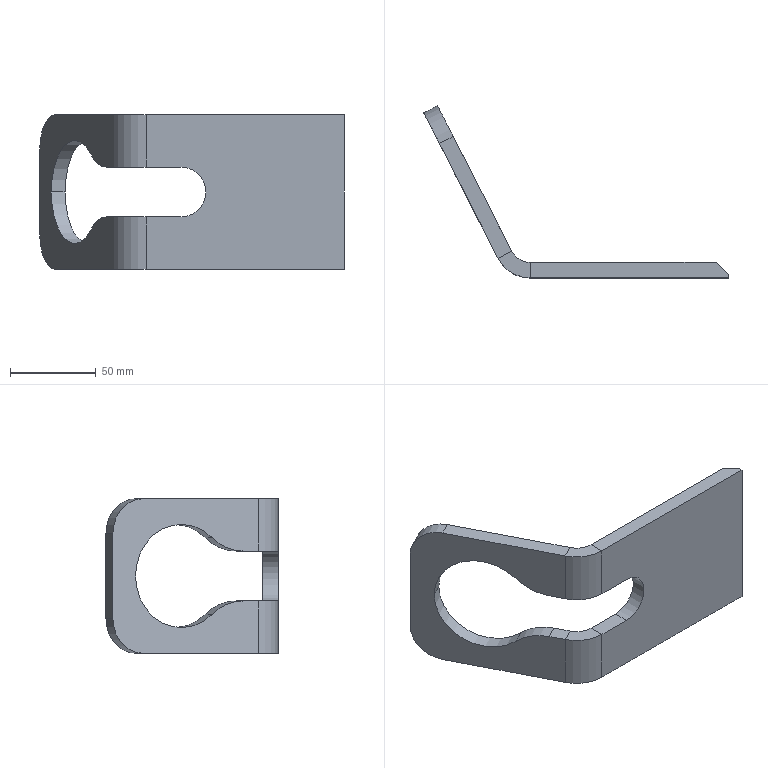Part | SolidWorks | features Fillet 2, Fold 2, ICE 2, UnFold 2, FlatPattern 1, SMBaseFlange 1, SheetMetal 1 | 1 solid | 30 faces | box 177 x 100.092 x 90 mm | volume 136681 mm3 | plane 19 | cylinder 11 | commonest cylinder face diameters 60 x4 24 x2 40 x2 42 x2 29 x1
STEP:
#1=CARTESIAN_POINT('',(-170.316,82.906,45.));
#2=VERTEX_POINT('',#1);
#3=CARTESIAN_POINT('',(-147.529,38.262,67.25));
#4=VERTEX_POINT('',#3);
#5=CARTESIAN_POINT('',(-156.678,56.185,45.));
#6=DIRECTION('',(0.8907,0.4546,0.));
#7=DIRECTION('',(-0.4546,0.8907,0.));
#8=AXIS2_PLACEMENT_3D('',#5,#6,#7);
#9=CIRCLE('',#8,30.);
#10=EDGE_CURVE('',#2,#4,#9,.T.);
#11=ORIENTED_EDGE('',*,*,#10,.F.);
#12=CARTESIAN_POINT('',(-162.3,86.997,45.));
#13=VERTEX_POINT('',#12);
#14=CARTESIAN_POINT('',(-170.316,82.906,45.));
#15=DIRECTION('',(0.8907,0.4546,0.));
#16=VECTOR('',#15,1000.);
#17=LINE('',#14,#16);
#18=EDGE_CURVE('',#2,#13,#17,.T.);
#19=ORIENTED_EDGE('',*,*,#18,.T.);
#20=CARTESIAN_POINT('',(-139.513,42.353,67.25));
#21=VERTEX_POINT('',#20);
#22=CARTESIAN_POINT('',(-148.662,60.277,45.));
#23=DIRECTION('',(0.8907,0.4546,0.));
#24=DIRECTION('',(-0.4546,0.8907,0.));
#25=AXIS2_PLACEMENT_3D('',#22,#23,#24);
#26=CIRCLE('',#25,30.);
#27=EDGE_CURVE('',#13,#21,#26,.T.);
#28=ORIENTED_EDGE('',*,*,#27,.T.);
#29=CARTESIAN_POINT('',(-147.529,38.262,67.25));
#30=DIRECTION('',(0.8907,0.4546,0.));
#31=VECTOR('',#30,1000.);
#32=LINE('',#29,#31);
#33=EDGE_CURVE('',#4,#21,#32,.T.);
#34=ORIENTED_EDGE('',*,*,#33,.F.);
#35=EDGE_LOOP('',(#11,#19,#28,#34));
#36=FACE_OUTER_BOUND('',#35,.T.);
#37=CARTESIAN_POINT('',(-156.678,56.185,45.));
#38=DIRECTION('',(0.8907,0.4546,0.));
#39=DIRECTION('',(-0.4546,0.8907,0.));
#40=AXIS2_PLACEMENT_3D('',#37,#38,#39);
#41=CYLINDRICAL_SURFACE('',#40,30.);
#42=ADVANCED_FACE('',(#36),#41,.F.);
#43=CARTESIAN_POINT('',(-133.846,11.453,59.5));
#44=VERTEX_POINT('',#43);
#45=CARTESIAN_POINT('',(-125.83,15.545,59.5));
#46=VERTEX_POINT('',#45);
#47=CARTESIAN_POINT('',(-133.846,11.453,59.5));
#48=DIRECTION('',(0.8907,0.4546,0.));
#49=VECTOR('',#48,1000.);
#50=LINE('',#47,#49);
#51=EDGE_CURVE('',#44,#46,#50,.T.);
#52=ORIENTED_EDGE('',*,*,#51,.F.);
#53=CARTESIAN_POINT('',(-138.381,20.338,59.5));
#54=VERTEX_POINT('',#53);
#55=CARTESIAN_POINT('',(-116.671,-22.195,59.5));
#56=DIRECTION('',(0.4546,-0.8907,0.));
#57=VECTOR('',#56,1000.);
#58=LINE('',#55,#57);
#59=EDGE_CURVE('',#54,#44,#58,.T.);
#60=ORIENTED_EDGE('',*,*,#59,.F.);
#61=CARTESIAN_POINT('',(-130.365,24.43,59.5));
#62=VERTEX_POINT('',#61);
#63=CARTESIAN_POINT('',(-138.381,20.338,59.5));
#64=DIRECTION('',(0.8907,0.4546,0.));
#65=VECTOR('',#64,1000.);
#66=LINE('',#63,#65);
#67=EDGE_CURVE('',#54,#62,#66,.T.);
#68=ORIENTED_EDGE('',*,*,#67,.T.);
#69=CARTESIAN_POINT('',(-108.655,-18.104,59.5));
#70=DIRECTION('',(0.4546,-0.8907,0.));
#71=VECTOR('',#70,1000.);
#72=LINE('',#69,#71);
#73=EDGE_CURVE('',#62,#46,#72,.T.);
#74=ORIENTED_EDGE('',*,*,#73,.T.);
#75=EDGE_LOOP('',(#52,#60,#68,#74));
#76=FACE_OUTER_BOUND('',#75,.T.);
#77=CARTESIAN_POINT('',(-116.671,-22.195,59.5));
#78=DIRECTION('',(0.,0.,1.));
#79=DIRECTION('',(0.4546,-0.8907,0.));
#80=AXIS2_PLACEMENT_3D('',#77,#78,#79);
#81=PLANE('',#80);
#82=ADVANCED_FACE('',(#76),#81,.F.);
#83=CARTESIAN_POINT('',(-125.83,15.545,30.5));
#84=VERTEX_POINT('',#83);
#85=CARTESIAN_POINT('',(-133.846,11.453,30.5));
#86=VERTEX_POINT('',#85);
#87=CARTESIAN_POINT('',(-125.83,15.545,30.5));
#88=DIRECTION('',(-0.8907,-0.4546,0.));
#89=VECTOR('',#88,1000.);
#90=LINE('',#87,#89);
#91=EDGE_CURVE('',#84,#86,#90,.T.);
#92=ORIENTED_EDGE('',*,*,#91,.F.);
#93=CARTESIAN_POINT('',(-130.365,24.43,30.5));
#94=VERTEX_POINT('',#93);
#95=CARTESIAN_POINT('',(-108.655,-18.104,30.5));
#96=DIRECTION('',(-0.4546,0.8907,0.));
#97=VECTOR('',#96,1000.);
#98=LINE('',#95,#97);
#99=EDGE_CURVE('',#84,#94,#98,.T.);
#100=ORIENTED_EDGE('',*,*,#99,.T.);
#101=CARTESIAN_POINT('',(-138.381,20.338,30.5));
#102=VERTEX_POINT('',#101);
#103=CARTESIAN_POINT('',(-138.381,20.338,30.5));
#104=DIRECTION('',(0.8907,0.4546,0.));
#105=VECTOR('',#104,1000.);
#106=LINE('',#103,#105);
#107=EDGE_CURVE('',#102,#94,#106,.T.);
#108=ORIENTED_EDGE('',*,*,#107,.F.);
#109=CARTESIAN_POINT('',(-116.671,-22.195,30.5));
#110=DIRECTION('',(-0.4546,0.8907,0.));
#111=VECTOR('',#110,1000.);
#112=LINE('',#109,#111);
#113=EDGE_CURVE('',#86,#102,#112,.T.);
#114=ORIENTED_EDGE('',*,*,#113,.F.);
#115=EDGE_LOOP('',(#92,#100,#108,#114));
#116=FACE_OUTER_BOUND('',#115,.T.);
#117=CARTESIAN_POINT('',(-116.671,-22.195,30.5));
#118=DIRECTION('',(0.,0.,-1.));
#119=DIRECTION('',(-0.4546,0.8907,0.));
#120=AXIS2_PLACEMENT_3D('',#117,#118,#119);
#121=PLANE('',#120);
#122=ADVANCED_FACE('',(#116),#121,.F.);
#123=CARTESIAN_POINT('',(-159.891,82.278,90.));
#124=VERTEX_POINT('',#123);
#125=CARTESIAN_POINT('',(-125.83,15.545,90.));
#126=VERTEX_POINT('',#125);
#127=CARTESIAN_POINT('',(-168.984,100.092,90.));
#128=DIRECTION('',(0.4546,-0.8907,0.));
#129=VECTOR('',#128,1000.);
#130=LINE('',#127,#129);
#131=EDGE_CURVE('',#124,#126,#130,.T.);
#132=ORIENTED_EDGE('',*,*,#131,.F.);
#133=CARTESIAN_POINT('',(-167.908,78.186,90.));
#134=VERTEX_POINT('',#133);
#135=CARTESIAN_POINT('',(-154.062,85.253,90.));
#136=DIRECTION('',(-0.8907,-0.4546,0.));
#137=VECTOR('',#136,1000.);
#138=LINE('',#135,#137);
#139=EDGE_CURVE('',#124,#134,#138,.T.);
#140=ORIENTED_EDGE('',*,*,#139,.T.);
#141=CARTESIAN_POINT('',(-133.846,11.453,90.));
#142=VERTEX_POINT('',#141);
#143=CARTESIAN_POINT('',(-177.,96.,90.));
#144=DIRECTION('',(0.4546,-0.8907,0.));
#145=VECTOR('',#144,1000.);
#146=LINE('',#143,#145);
#147=EDGE_CURVE('',#134,#142,#146,.T.);
#148=ORIENTED_EDGE('',*,*,#147,.T.);
#149=CARTESIAN_POINT('',(-133.846,11.453,90.));
#150=DIRECTION('',(0.8907,0.4546,0.));
#151=VECTOR('',#150,1000.);
#152=LINE('',#149,#151);
#153=EDGE_CURVE('',#142,#126,#152,.T.);
#154=ORIENTED_EDGE('',*,*,#153,.T.);
#155=EDGE_LOOP('',(#132,#140,#148,#154));
#156=FACE_OUTER_BOUND('',#155,.T.);
#157=CARTESIAN_POINT('',(-115.141,9.,90.));
#158=DIRECTION('',(0.,0.,1.));
#159=DIRECTION('',(1.,0.,0.));
#160=AXIS2_PLACEMENT_3D('',#157,#158,#159);
#161=PLANE('',#160);
#162=ADVANCED_FACE('',(#156),#161,.T.);
#163=ORIENTED_EDGE('',*,*,#99,.F.);
#164=CARTESIAN_POINT('',(-125.83,15.545,0.));
#165=VERTEX_POINT('',#164);
#166=CARTESIAN_POINT('',(-125.83,15.545,90.));
#167=DIRECTION('',(0.,0.,-1.));
#168=VECTOR('',#167,1000.);
#169=LINE('',#166,#168);
#170=EDGE_CURVE('',#84,#165,#169,.T.);
#171=ORIENTED_EDGE('',*,*,#170,.T.);
#172=CARTESIAN_POINT('',(-159.891,82.278,0.));
#173=VERTEX_POINT('',#172);
#174=CARTESIAN_POINT('',(-168.984,100.092,0.));
#175=DIRECTION('',(0.4546,-0.8907,0.));
#176=VECTOR('',#175,1000.);
#177=LINE('',#174,#176);
#178=EDGE_CURVE('',#173,#165,#177,.T.);
#179=ORIENTED_EDGE('',*,*,#178,.F.);
#180=CARTESIAN_POINT('',(-168.984,100.092,20.));
#181=VERTEX_POINT('',#180);
#182=CARTESIAN_POINT('',(-159.891,82.278,20.));
#183=DIRECTION('',(0.8907,0.4546,0.));
#184=DIRECTION('',(-0.4546,0.8907,0.));
#185=AXIS2_PLACEMENT_3D('',#182,#183,#184);
#186=CIRCLE('',#185,20.);
#187=EDGE_CURVE('',#173,#181,#186,.T.);
#188=ORIENTED_EDGE('',*,*,#187,.T.);
#189=CARTESIAN_POINT('',(-168.984,100.092,70.));
#190=VERTEX_POINT('',#189);
#191=CARTESIAN_POINT('',(-168.984,100.092,90.));
#192=DIRECTION('',(0.,0.,-1.));
#193=VECTOR('',#192,1000.);
#194=LINE('',#191,#193);
#195=EDGE_CURVE('',#190,#181,#194,.T.);
#196=ORIENTED_EDGE('',*,*,#195,.F.);
#197=CARTESIAN_POINT('',(-159.891,82.278,70.));
#198=DIRECTION('',(0.8907,0.4546,0.));
#199=DIRECTION('',(-0.4546,0.8907,0.));
#200=AXIS2_PLACEMENT_3D('',#197,#198,#199);
#201=CIRCLE('',#200,20.);
#202=EDGE_CURVE('',#190,#124,#201,.T.);
#203=ORIENTED_EDGE('',*,*,#202,.T.);
#204=ORIENTED_EDGE('',*,*,#131,.T.);
#205=CARTESIAN_POINT('',(-125.83,15.545,90.));
#206=DIRECTION('',(0.,0.,-1.));
#207=VECTOR('',#206,1000.);
#208=LINE('',#205,#207);
#209=EDGE_CURVE('',#126,#46,#208,.T.);
#210=ORIENTED_EDGE('',*,*,#209,.T.);
#211=ORIENTED_EDGE('',*,*,#73,.F.);
#212=CARTESIAN_POINT('',(-130.365,24.43,89.5));
#213=DIRECTION('',(-0.8907,-0.4546,0.));
#214=DIRECTION('',(-0.4546,0.8907,0.));
#215=AXIS2_PLACEMENT_3D('',#212,#213,#214);
#216=CIRCLE('',#215,30.);
#217=EDGE_CURVE('',#21,#62,#216,.T.);
#218=ORIENTED_EDGE('',*,*,#217,.F.);
#219=ORIENTED_EDGE('',*,*,#27,.F.);
#220=CARTESIAN_POINT('',(-139.513,42.353,22.75));
#221=VERTEX_POINT('',#220);
#222=CARTESIAN_POINT('',(-148.662,60.277,45.));
#223=DIRECTION('',(0.8907,0.4546,0.));
#224=DIRECTION('',(-0.4546,0.8907,0.));
#225=AXIS2_PLACEMENT_3D('',#222,#223,#224);
#226=CIRCLE('',#225,30.);
#227=EDGE_CURVE('',#221,#13,#226,.T.);
#228=ORIENTED_EDGE('',*,*,#227,.F.);
#229=CARTESIAN_POINT('',(-130.365,24.43,0.5));
#230=DIRECTION('',(-0.8907,-0.4546,0.));
#231=DIRECTION('',(0.4546,-0.8907,0.));
#232=AXIS2_PLACEMENT_3D('',#229,#230,#231);
#233=CIRCLE('',#232,30.);
#234=EDGE_CURVE('',#94,#221,#233,.T.);
#235=ORIENTED_EDGE('',*,*,#234,.F.);
#236=EDGE_LOOP('',(#163,#171,#179,#188,#196,#203,#204,#210,#211,#218,#219,#228,#235));
#237=FACE_OUTER_BOUND('',#236,.T.);
#238=CARTESIAN_POINT('',(-168.984,100.092,90.));
#239=DIRECTION('',(0.8907,0.4546,0.));
#240=DIRECTION('',(-0.4546,0.8907,0.));
#241=AXIS2_PLACEMENT_3D('',#238,#239,#240);
#242=PLANE('',#241);
#243=ADVANCED_FACE('',(#237),#242,.T.);
#244=ORIENTED_EDGE('',*,*,#195,.T.);
#245=CARTESIAN_POINT('',(-177.,96.,20.));
#246=VERTEX_POINT('',#245);
#247=CARTESIAN_POINT('',(-177.,96.,20.));
#248=DIRECTION('',(-0.8907,-0.4546,0.));
#249=VECTOR('',#248,1000.);
#250=LINE('',#247,#249);
#251=EDGE_CURVE('',#181,#246,#250,.T.);
#252=ORIENTED_EDGE('',*,*,#251,.T.);
#253=CARTESIAN_POINT('',(-177.,96.,70.));
#254=VERTEX_POINT('',#253);
#255=CARTESIAN_POINT('',(-177.,96.,90.));
#256=DIRECTION('',(0.,0.,-1.));
#257=VECTOR('',#256,1000.);
#258=LINE('',#255,#257);
#259=EDGE_CURVE('',#254,#246,#258,.T.);
#260=ORIENTED_EDGE('',*,*,#259,.F.);
#261=CARTESIAN_POINT('',(-177.,96.,70.));
#262=DIRECTION('',(0.8907,0.4546,0.));
#263=VECTOR('',#262,1000.);
#264=LINE('',#261,#263);
#265=EDGE_CURVE('',#254,#190,#264,.T.);
#266=ORIENTED_EDGE('',*,*,#265,.T.);
#267=EDGE_LOOP('',(#244,#252,#260,#266));
#268=FACE_OUTER_BOUND('',#267,.T.);
#269=CARTESIAN_POINT('',(-177.,96.,90.));
#270=DIRECTION('',(-0.4546,0.8907,0.));
#271=DIRECTION('',(-0.8907,-0.4546,0.));
#272=AXIS2_PLACEMENT_3D('',#269,#270,#271);
#273=PLANE('',#272);
#274=ADVANCED_FACE('',(#268),#273,.T.);
#275=CARTESIAN_POINT('',(-133.846,11.453,0.));
#276=VERTEX_POINT('',#275);
#277=CARTESIAN_POINT('',(-133.846,11.453,90.));
#278=DIRECTION('',(0.,0.,-1.));
#279=VECTOR('',#278,1000.);
#280=LINE('',#277,#279);
#281=EDGE_CURVE('',#86,#276,#280,.T.);
#282=ORIENTED_EDGE('',*,*,#281,.F.);
#283=ORIENTED_EDGE('',*,*,#113,.T.);
#284=CARTESIAN_POINT('',(-147.529,38.262,22.75));
#285=VERTEX_POINT('',#284);
#286=CARTESIAN_POINT('',(-138.381,20.338,0.5));
#287=DIRECTION('',(-0.8907,-0.4546,0.));
#288=DIRECTION('',(0.4546,-0.8907,0.));
#289=AXIS2_PLACEMENT_3D('',#286,#287,#288);
#290=CIRCLE('',#289,30.);
#291=EDGE_CURVE('',#102,#285,#290,.T.);
#292=ORIENTED_EDGE('',*,*,#291,.T.);
#293=CARTESIAN_POINT('',(-156.678,56.185,45.));
#294=DIRECTION('',(0.8907,0.4546,0.));
#295=DIRECTION('',(-0.4546,0.8907,0.));
#296=AXIS2_PLACEMENT_3D('',#293,#294,#295);
#297=CIRCLE('',#296,30.);
#298=EDGE_CURVE('',#285,#2,#297,.T.);
#299=ORIENTED_EDGE('',*,*,#298,.T.);
#300=ORIENTED_EDGE('',*,*,#10,.T.);
#301=CARTESIAN_POINT('',(-138.381,20.338,89.5));
#302=DIRECTION('',(-0.8907,-0.4546,0.));
#303=DIRECTION('',(-0.4546,0.8907,0.));
#304=AXIS2_PLACEMENT_3D('',#301,#302,#303);
#305=CIRCLE('',#304,30.);
#306=EDGE_CURVE('',#4,#54,#305,.T.);
#307=ORIENTED_EDGE('',*,*,#306,.T.);
#308=ORIENTED_EDGE('',*,*,#59,.T.);
#309=CARTESIAN_POINT('',(-133.846,11.453,90.));
#310=DIRECTION('',(0.,0.,-1.));
#311=VECTOR('',#310,1000.);
#312=LINE('',#309,#311);
#313=EDGE_CURVE('',#142,#44,#312,.T.);
#314=ORIENTED_EDGE('',*,*,#313,.F.);
#315=ORIENTED_EDGE('',*,*,#147,.F.);
#316=CARTESIAN_POINT('',(-167.908,78.186,70.));
#317=DIRECTION('',(-0.8907,-0.4546,0.));
#318=DIRECTION('',(-0.4546,0.8907,0.));
#319=AXIS2_PLACEMENT_3D('',#316,#317,#318);
#320=CIRCLE('',#319,20.);
#321=EDGE_CURVE('',#134,#254,#320,.T.);
#322=ORIENTED_EDGE('',*,*,#321,.T.);
#323=ORIENTED_EDGE('',*,*,#259,.T.);
#324=CARTESIAN_POINT('',(-167.908,78.186,0.));
#325=VERTEX_POINT('',#324);
#326=CARTESIAN_POINT('',(-167.908,78.186,20.));
#327=DIRECTION('',(-0.8907,-0.4546,0.));
#328=DIRECTION('',(-0.4546,0.8907,0.));
#329=AXIS2_PLACEMENT_3D('',#326,#327,#328);
#330=CIRCLE('',#329,20.);
#331=EDGE_CURVE('',#246,#325,#330,.T.);
#332=ORIENTED_EDGE('',*,*,#331,.T.);
#333=CARTESIAN_POINT('',(-177.,96.,0.));
#334=DIRECTION('',(0.4546,-0.8907,0.));
#335=VECTOR('',#334,1000.);
#336=LINE('',#333,#335);
#337=EDGE_CURVE('',#325,#276,#336,.T.);
#338=ORIENTED_EDGE('',*,*,#337,.T.);
#339=EDGE_LOOP('',(#282,#283,#292,#299,#300,#307,#308,#314,#315,#322,#323,#332,#338));
#340=FACE_OUTER_BOUND('',#339,.T.);
#341=CARTESIAN_POINT('',(-177.,96.,90.));
#342=DIRECTION('',(0.8907,0.4546,0.));
#343=DIRECTION('',(-0.4546,0.8907,0.));
#344=AXIS2_PLACEMENT_3D('',#341,#342,#343);
#345=PLANE('',#344);
#346=ADVANCED_FACE('',(#340),#345,.F.);
#347=ORIENTED_EDGE('',*,*,#337,.F.);
#348=CARTESIAN_POINT('',(-159.891,82.278,0.));
#349=DIRECTION('',(0.8907,0.4546,0.));
#350=VECTOR('',#349,1000.);
#351=LINE('',#348,#350);
#352=EDGE_CURVE('',#325,#173,#351,.T.);
#353=ORIENTED_EDGE('',*,*,#352,.T.);
#354=ORIENTED_EDGE('',*,*,#178,.T.);
#355=CARTESIAN_POINT('',(-125.83,15.545,0.));
#356=DIRECTION('',(-0.8907,-0.4546,0.));
#357=VECTOR('',#356,1000.);
#358=LINE('',#355,#357);
#359=EDGE_CURVE('',#165,#276,#358,.T.);
#360=ORIENTED_EDGE('',*,*,#359,.T.);
#361=EDGE_LOOP('',(#347,#353,#354,#360));
#362=FACE_OUTER_BOUND('',#361,.T.);
#363=CARTESIAN_POINT('',(-115.141,21.,0.));
#364=DIRECTION('',(0.,0.,1.));
#365=DIRECTION('',(1.,0.,0.));
#366=AXIS2_PLACEMENT_3D('',#363,#364,#365);
#367=PLANE('',#366);
#368=ADVANCED_FACE('',(#362),#367,.F.);
#369=ORIENTED_EDGE('',*,*,#321,.F.);
#370=ORIENTED_EDGE('',*,*,#139,.F.);
#371=ORIENTED_EDGE('',*,*,#202,.F.);
#372=ORIENTED_EDGE('',*,*,#265,.F.);
#373=EDGE_LOOP('',(#369,#370,#371,#372));
#374=FACE_OUTER_BOUND('',#373,.T.);
#375=CARTESIAN_POINT('',(-167.908,78.186,70.));
#376=DIRECTION('',(0.8907,0.4546,0.));
#377=DIRECTION('',(-0.4546,0.8907,0.));
#378=AXIS2_PLACEMENT_3D('',#375,#376,#377);
#379=CYLINDRICAL_SURFACE('',#378,20.);
#380=ADVANCED_FACE('',(#374),#379,.T.);
#381=ORIENTED_EDGE('',*,*,#331,.F.);
#382=ORIENTED_EDGE('',*,*,#251,.F.);
#383=ORIENTED_EDGE('',*,*,#187,.F.);
#384=ORIENTED_EDGE('',*,*,#352,.F.);
#385=EDGE_LOOP('',(#381,#382,#383,#384));
#386=FACE_OUTER_BOUND('',#385,.T.);
#387=CARTESIAN_POINT('',(-149.203,87.733,20.));
#388=DIRECTION('',(-0.8907,-0.4546,0.));
#389=DIRECTION('',(0.4546,-0.8907,0.));
#390=AXIS2_PLACEMENT_3D('',#387,#388,#389);
#391=CYLINDRICAL_SURFACE('',#390,20.);
#392=ADVANCED_FACE('',(#386),#391,.T.);
#393=ORIENTED_EDGE('',*,*,#217,.T.);
#394=ORIENTED_EDGE('',*,*,#67,.F.);
#395=ORIENTED_EDGE('',*,*,#306,.F.);
#396=ORIENTED_EDGE('',*,*,#33,.T.);
#397=EDGE_LOOP('',(#393,#394,#395,#396));
#398=FACE_OUTER_BOUND('',#397,.T.);
#399=CARTESIAN_POINT('',(-138.381,20.338,89.5));
#400=DIRECTION('',(0.8907,0.4546,0.));
#401=DIRECTION('',(-0.4546,0.8907,0.));
#402=AXIS2_PLACEMENT_3D('',#399,#400,#401);
#403=CYLINDRICAL_SURFACE('',#402,30.);
#404=ADVANCED_FACE('',(#398),#403,.T.);
#405=ORIENTED_EDGE('',*,*,#18,.F.);
#406=ORIENTED_EDGE('',*,*,#298,.F.);
#407=CARTESIAN_POINT('',(-147.529,38.262,22.75));
#408=DIRECTION('',(0.8907,0.4546,0.));
#409=VECTOR('',#408,1000.);
#410=LINE('',#407,#409);
#411=EDGE_CURVE('',#285,#221,#410,.T.);
#412=ORIENTED_EDGE('',*,*,#411,.T.);
#413=ORIENTED_EDGE('',*,*,#227,.T.);
#414=EDGE_LOOP('',(#405,#406,#412,#413));
#415=FACE_OUTER_BOUND('',#414,.T.);
#416=CARTESIAN_POINT('',(-156.678,56.185,45.));
#417=DIRECTION('',(0.8907,0.4546,0.));
#418=DIRECTION('',(-0.4546,0.8907,0.));
#419=AXIS2_PLACEMENT_3D('',#416,#417,#418);
#420=CYLINDRICAL_SURFACE('',#419,30.);
#421=ADVANCED_FACE('',(#415),#420,.F.);
#422=ORIENTED_EDGE('',*,*,#234,.T.);
#423=ORIENTED_EDGE('',*,*,#411,.F.);
#424=ORIENTED_EDGE('',*,*,#291,.F.);
#425=ORIENTED_EDGE('',*,*,#107,.T.);
#426=EDGE_LOOP('',(#422,#423,#424,#425));
#427=FACE_OUTER_BOUND('',#426,.T.);
#428=CARTESIAN_POINT('',(-138.381,20.338,0.5));
#429=DIRECTION('',(0.8907,0.4546,0.));
#430=DIRECTION('',(-0.4546,0.8907,0.));
#431=AXIS2_PLACEMENT_3D('',#428,#429,#430);
#432=CYLINDRICAL_SURFACE('',#431,30.);
#433=ADVANCED_FACE('',(#427),#432,.T.);
#434=CARTESIAN_POINT('',(0.,2.,0.));
#435=VERTEX_POINT('',#434);
#436=CARTESIAN_POINT('',(0.,2.,90.));
#437=VERTEX_POINT('',#436);
#438=CARTESIAN_POINT('',(0.,2.,-22.));
#439=DIRECTION('',(0.,0.,1.));
#440=VECTOR('',#439,1000.);
#441=LINE('',#438,#440);
#442=EDGE_CURVE('',#435,#437,#441,.T.);
#443=ORIENTED_EDGE('',*,*,#442,.T.);
#444=CARTESIAN_POINT('',(0.,0.,90.));
#445=VERTEX_POINT('',#444);
#446=CARTESIAN_POINT('',(0.,9.,90.));
#447=DIRECTION('',(0.,-1.,0.));
#448=VECTOR('',#447,1000.);
#449=LINE('',#446,#448);
#450=EDGE_CURVE('',#437,#445,#449,.T.);
#451=ORIENTED_EDGE('',*,*,#450,.T.);
#452=CARTESIAN_POINT('',(0.,0.,0.));
#453=VERTEX_POINT('',#452);
#454=CARTESIAN_POINT('',(0.,0.,90.));
#455=DIRECTION('',(0.,0.,-1.));
#456=VECTOR('',#455,1000.);
#457=LINE('',#454,#456);
#458=EDGE_CURVE('',#445,#453,#457,.T.);
#459=ORIENTED_EDGE('',*,*,#458,.T.);
#460=CARTESIAN_POINT('',(0.,9.,0.));
#461=DIRECTION('',(0.,-1.,0.));
#462=VECTOR('',#461,1000.);
#463=LINE('',#460,#462);
#464=EDGE_CURVE('',#435,#453,#463,.T.);
#465=ORIENTED_EDGE('',*,*,#464,.F.);
#466=EDGE_LOOP('',(#443,#451,#459,#465));
#467=FACE_OUTER_BOUND('',#466,.T.);
#468=CARTESIAN_POINT('',(0.,9.,90.));
#469=DIRECTION('',(1.,0.,0.));
#470=DIRECTION('',(0.,1.,0.));
#471=AXIS2_PLACEMENT_3D('',#468,#469,#470);
#472=PLANE('',#471);
#473=ADVANCED_FACE('',(#467),#472,.T.);
#474=CARTESIAN_POINT('',(-7.,9.,0.));
#475=VERTEX_POINT('',#474);
#476=CARTESIAN_POINT('',(-69.687,71.687,0.));
#477=DIRECTION('',(-0.7071,0.7071,0.));
#478=VECTOR('',#477,1000.);
#479=LINE('',#476,#478);
#480=EDGE_CURVE('',#435,#475,#479,.T.);
#481=ORIENTED_EDGE('',*,*,#480,.T.);
#482=CARTESIAN_POINT('',(-7.,9.,90.));
#483=VERTEX_POINT('',#482);
#484=CARTESIAN_POINT('',(-7.,9.,-22.));
#485=DIRECTION('',(0.,0.,1.));
#486=VECTOR('',#485,1000.);
#487=LINE('',#484,#486);
#488=EDGE_CURVE('',#475,#483,#487,.T.);
#489=ORIENTED_EDGE('',*,*,#488,.T.);
#490=CARTESIAN_POINT('',(-7.,9.,90.));
#491=DIRECTION('',(0.7071,-0.7071,0.));
#492=VECTOR('',#491,1000.);
#493=LINE('',#490,#492);
#494=EDGE_CURVE('',#483,#437,#493,.T.);
#495=ORIENTED_EDGE('',*,*,#494,.T.);
#496=ORIENTED_EDGE('',*,*,#442,.F.);
#497=EDGE_LOOP('',(#481,#489,#495,#496));
#498=FACE_OUTER_BOUND('',#497,.T.);
#499=CARTESIAN_POINT('',(-7.,9.,-22.));
#500=DIRECTION('',(-0.7071,-0.7071,0.));
#501=DIRECTION('',(0.7071,-0.7071,0.));
#502=AXIS2_PLACEMENT_3D('',#499,#500,#501);
#503=PLANE('',#502);
#504=ADVANCED_FACE('',(#498),#503,.F.);
#505=CARTESIAN_POINT('',(-95.,9.,59.5));
#506=VERTEX_POINT('',#505);
#507=CARTESIAN_POINT('',(-95.,9.,30.5));
#508=VERTEX_POINT('',#507);
#509=CARTESIAN_POINT('',(-95.,9.,45.));
#510=DIRECTION('',(0.,1.,0.));
#511=DIRECTION('',(-1.,0.,0.));
#512=AXIS2_PLACEMENT_3D('',#509,#510,#511);
#513=CIRCLE('',#512,14.5);
#514=EDGE_CURVE('',#506,#508,#513,.T.);
#515=ORIENTED_EDGE('',*,*,#514,.T.);
#516=CARTESIAN_POINT('',(-95.,0.,30.5));
#517=VERTEX_POINT('',#516);
#518=CARTESIAN_POINT('',(-95.,0.,30.5));
#519=DIRECTION('',(0.,1.,0.));
#520=VECTOR('',#519,1000.);
#521=LINE('',#518,#520);
#522=EDGE_CURVE('',#517,#508,#521,.T.);
#523=ORIENTED_EDGE('',*,*,#522,.F.);
#524=CARTESIAN_POINT('',(-95.,0.,59.5));
#525=VERTEX_POINT('',#524);
#526=CARTESIAN_POINT('',(-95.,0.,45.));
#527=DIRECTION('',(0.,1.,0.));
#528=DIRECTION('',(-1.,0.,0.));
#529=AXIS2_PLACEMENT_3D('',#526,#527,#528);
#530=CIRCLE('',#529,14.5);
#531=EDGE_CURVE('',#525,#517,#530,.T.);
#532=ORIENTED_EDGE('',*,*,#531,.F.);
#533=CARTESIAN_POINT('',(-95.,0.,59.5));
#534=DIRECTION('',(0.,1.,0.));
#535=VECTOR('',#534,1000.);
#536=LINE('',#533,#535);
#537=EDGE_CURVE('',#525,#506,#536,.T.);
#538=ORIENTED_EDGE('',*,*,#537,.T.);
#539=EDGE_LOOP('',(#515,#523,#532,#538));
#540=FACE_OUTER_BOUND('',#539,.T.);
#541=CARTESIAN_POINT('',(-95.,0.,45.));
#542=DIRECTION('',(0.,1.,0.));
#543=DIRECTION('',(-1.,0.,0.));
#544=AXIS2_PLACEMENT_3D('',#541,#542,#543);
#545=CYLINDRICAL_SURFACE('',#544,14.5);
#546=ADVANCED_FACE('',(#540),#545,.F.);
#547=CARTESIAN_POINT('',(-115.141,9.,30.5));
#548=VERTEX_POINT('',#547);
#549=CARTESIAN_POINT('',(-95.,9.,30.5));
#550=DIRECTION('',(-1.,0.,0.));
#551=VECTOR('',#550,1000.);
#552=LINE('',#549,#551);
#553=EDGE_CURVE('',#508,#548,#552,.T.);
#554=ORIENTED_EDGE('',*,*,#553,.F.);
#555=ORIENTED_EDGE('',*,*,#514,.F.);
#556=CARTESIAN_POINT('',(-115.141,9.,59.5));
#557=VERTEX_POINT('',#556);
#558=CARTESIAN_POINT('',(-95.,9.,59.5));
#559=DIRECTION('',(1.,0.,0.));
#560=VECTOR('',#559,1000.);
#561=LINE('',#558,#560);
#562=EDGE_CURVE('',#557,#506,#561,.T.);
#563=ORIENTED_EDGE('',*,*,#562,.F.);
#564=CARTESIAN_POINT('',(-115.141,9.,90.));
#565=VERTEX_POINT('',#564);
#566=CARTESIAN_POINT('',(-115.141,9.,90.));
#567=DIRECTION('',(0.,0.,-1.));
#568=VECTOR('',#567,1000.);
#569=LINE('',#566,#568);
#570=EDGE_CURVE('',#565,#557,#569,.T.);
#571=ORIENTED_EDGE('',*,*,#570,.F.);
#572=CARTESIAN_POINT('',(0.,9.,90.));
#573=DIRECTION('',(1.,0.,0.));
#574=VECTOR('',#573,1000.);
#575=LINE('',#572,#574);
#576=EDGE_CURVE('',#565,#483,#575,.T.);
#577=ORIENTED_EDGE('',*,*,#576,.T.);
#578=ORIENTED_EDGE('',*,*,#488,.F.);
#579=CARTESIAN_POINT('',(-115.141,9.,0.));
#580=VERTEX_POINT('',#579);
#581=CARTESIAN_POINT('',(0.,9.,0.));
#582=DIRECTION('',(1.,0.,0.));
#583=VECTOR('',#582,1000.);
#584=LINE('',#581,#583);
#585=EDGE_CURVE('',#580,#475,#584,.T.);
#586=ORIENTED_EDGE('',*,*,#585,.F.);
#587=CARTESIAN_POINT('',(-115.141,9.,90.));
#588=DIRECTION('',(0.,0.,-1.));
#589=VECTOR('',#588,1000.);
#590=LINE('',#587,#589);
#591=EDGE_CURVE('',#548,#580,#590,.T.);
#592=ORIENTED_EDGE('',*,*,#591,.F.);
#593=EDGE_LOOP('',(#554,#555,#563,#571,#577,#578,#586,#592));
#594=FACE_OUTER_BOUND('',#593,.T.);
#595=CARTESIAN_POINT('',(0.,9.,90.));
#596=DIRECTION('',(0.,1.,0.));
#597=DIRECTION('',(-1.,0.,0.));
#598=AXIS2_PLACEMENT_3D('',#595,#596,#597);
#599=PLANE('',#598);
#600=ADVANCED_FACE('',(#594),#599,.T.);
#601=CARTESIAN_POINT('',(-115.141,0.,30.5));
#602=VERTEX_POINT('',#601);
#603=CARTESIAN_POINT('',(-115.141,0.,30.5));
#604=DIRECTION('',(0.,1.,0.));
#605=VECTOR('',#604,1000.);
#606=LINE('',#603,#605);
#607=EDGE_CURVE('',#602,#548,#606,.T.);
#608=ORIENTED_EDGE('',*,*,#607,.F.);
#609=CARTESIAN_POINT('',(-95.,0.,30.5));
#610=DIRECTION('',(-1.,0.,0.));
#611=VECTOR('',#610,1000.);
#612=LINE('',#609,#611);
#613=EDGE_CURVE('',#517,#602,#612,.T.);
#614=ORIENTED_EDGE('',*,*,#613,.F.);
#615=ORIENTED_EDGE('',*,*,#522,.T.);
#616=ORIENTED_EDGE('',*,*,#553,.T.);
#617=EDGE_LOOP('',(#608,#614,#615,#616));
#618=FACE_OUTER_BOUND('',#617,.T.);
#619=CARTESIAN_POINT('',(-95.,0.,30.5));
#620=DIRECTION('',(0.,0.,-1.));
#621=DIRECTION('',(-1.,0.,0.));
#622=AXIS2_PLACEMENT_3D('',#619,#620,#621);
#623=PLANE('',#622);
#624=ADVANCED_FACE('',(#618),#623,.F.);
#625=ORIENTED_EDGE('',*,*,#531,.T.);
#626=ORIENTED_EDGE('',*,*,#613,.T.);
#627=CARTESIAN_POINT('',(-115.141,0.,0.));
#628=VERTEX_POINT('',#627);
#629=CARTESIAN_POINT('',(-115.141,0.,90.));
#630=DIRECTION('',(0.,0.,-1.));
#631=VECTOR('',#630,1000.);
#632=LINE('',#629,#631);
#633=EDGE_CURVE('',#602,#628,#632,.T.);
#634=ORIENTED_EDGE('',*,*,#633,.T.);
#635=CARTESIAN_POINT('',(0.,0.,0.));
#636=DIRECTION('',(1.,0.,0.));
#637=VECTOR('',#636,1000.);
#638=LINE('',#635,#637);
#639=EDGE_CURVE('',#628,#453,#638,.T.);
#640=ORIENTED_EDGE('',*,*,#639,.T.);
#641=ORIENTED_EDGE('',*,*,#458,.F.);
#642=CARTESIAN_POINT('',(-115.141,0.,90.));
#643=VERTEX_POINT('',#642);
#644=CARTESIAN_POINT('',(0.,0.,90.));
#645=DIRECTION('',(1.,0.,0.));
#646=VECTOR('',#645,1000.);
#647=LINE('',#644,#646);
#648=EDGE_CURVE('',#643,#445,#647,.T.);
#649=ORIENTED_EDGE('',*,*,#648,.F.);
#650=CARTESIAN_POINT('',(-115.141,0.,59.5));
#651=VERTEX_POINT('',#650);
#652=CARTESIAN_POINT('',(-115.141,0.,90.));
#653=DIRECTION('',(0.,0.,-1.));
#654=VECTOR('',#653,1000.);
#655=LINE('',#652,#654);
#656=EDGE_CURVE('',#643,#651,#655,.T.);
#657=ORIENTED_EDGE('',*,*,#656,.T.);
#658=CARTESIAN_POINT('',(-95.,0.,59.5));
#659=DIRECTION('',(1.,0.,0.));
#660=VECTOR('',#659,1000.);
#661=LINE('',#658,#660);
#662=EDGE_CURVE('',#651,#525,#661,.T.);
#663=ORIENTED_EDGE('',*,*,#662,.T.);
#664=EDGE_LOOP('',(#625,#626,#634,#640,#641,#649,#657,#663));
#665=FACE_OUTER_BOUND('',#664,.T.);
#666=CARTESIAN_POINT('',(0.,0.,90.));
#667=DIRECTION('',(0.,1.,0.));
#668=DIRECTION('',(-1.,0.,0.));
#669=AXIS2_PLACEMENT_3D('',#666,#667,#668);
#670=PLANE('',#669);
#671=ADVANCED_FACE('',(#665),#670,.F.);
#672=ORIENTED_EDGE('',*,*,#480,.F.);
#673=ORIENTED_EDGE('',*,*,#464,.T.);
#674=ORIENTED_EDGE('',*,*,#639,.F.);
#675=CARTESIAN_POINT('',(-115.141,0.,0.));
#676=DIRECTION('',(0.,1.,0.));
#677=VECTOR('',#676,1000.);
#678=LINE('',#675,#677);
#679=EDGE_CURVE('',#628,#580,#678,.T.);
#680=ORIENTED_EDGE('',*,*,#679,.T.);
#681=ORIENTED_EDGE('',*,*,#585,.T.);
#682=EDGE_LOOP('',(#672,#673,#674,#680,#681));
#683=FACE_OUTER_BOUND('',#682,.T.);
#684=CARTESIAN_POINT('',(-125.83,15.545,0.));
#685=DIRECTION('',(0.,0.,-1.));
#686=DIRECTION('',(-1.,0.,0.));
#687=AXIS2_PLACEMENT_3D('',#684,#685,#686);
#688=PLANE('',#687);
#689=ADVANCED_FACE('',(#683),#688,.T.);
#690=ORIENTED_EDGE('',*,*,#494,.F.);
#691=ORIENTED_EDGE('',*,*,#576,.F.);
#692=CARTESIAN_POINT('',(-115.141,9.,90.));
#693=DIRECTION('',(0.,-1.,0.));
#694=VECTOR('',#693,1000.);
#695=LINE('',#692,#694);
#696=EDGE_CURVE('',#565,#643,#695,.T.);
#697=ORIENTED_EDGE('',*,*,#696,.T.);
#698=ORIENTED_EDGE('',*,*,#648,.T.);
#699=ORIENTED_EDGE('',*,*,#450,.F.);
#700=EDGE_LOOP('',(#690,#691,#697,#698,#699));
#701=FACE_OUTER_BOUND('',#700,.T.);
#702=CARTESIAN_POINT('',(-115.141,21.,90.));
#703=DIRECTION('',(0.,0.,1.));
#704=DIRECTION('',(1.,0.,0.));
#705=AXIS2_PLACEMENT_3D('',#702,#703,#704);
#706=PLANE('',#705);
#707=ADVANCED_FACE('',(#701),#706,.T.);
#708=CARTESIAN_POINT('',(-115.141,9.,59.5));
#709=DIRECTION('',(0.,-1.,0.));
#710=VECTOR('',#709,1000.);
#711=LINE('',#708,#710);
#712=EDGE_CURVE('',#557,#651,#711,.T.);
#713=ORIENTED_EDGE('',*,*,#712,.F.);
#714=ORIENTED_EDGE('',*,*,#562,.T.);
#715=ORIENTED_EDGE('',*,*,#537,.F.);
#716=ORIENTED_EDGE('',*,*,#662,.F.);
#717=EDGE_LOOP('',(#713,#714,#715,#716));
#718=FACE_OUTER_BOUND('',#717,.T.);
#719=CARTESIAN_POINT('',(-95.,0.,59.5));
#720=DIRECTION('',(0.,0.,1.));
#721=DIRECTION('',(1.,0.,0.));
#722=AXIS2_PLACEMENT_3D('',#719,#720,#721);
#723=PLANE('',#722);
#724=ADVANCED_FACE('',(#718),#723,.F.);
#725=ORIENTED_EDGE('',*,*,#91,.T.);
#726=CARTESIAN_POINT('',(-115.141,21.,30.5));
#727=DIRECTION('',(0.,0.,1.));
#728=DIRECTION('',(1.,0.,0.));
#729=AXIS2_PLACEMENT_3D('',#726,#727,#728);
#730=CIRCLE('',#729,21.);
#731=EDGE_CURVE('',#86,#602,#730,.T.);
#732=ORIENTED_EDGE('',*,*,#731,.T.);
#733=ORIENTED_EDGE('',*,*,#607,.T.);
#734=CARTESIAN_POINT('',(-115.141,21.,30.5));
#735=DIRECTION('',(0.,0.,1.));
#736=DIRECTION('',(-1.,0.,0.));
#737=AXIS2_PLACEMENT_3D('',#734,#735,#736);
#738=CIRCLE('',#737,12.);
#739=EDGE_CURVE('',#84,#548,#738,.T.);
#740=ORIENTED_EDGE('',*,*,#739,.F.);
#741=EDGE_LOOP('',(#725,#732,#733,#740));
#742=FACE_OUTER_BOUND('',#741,.T.);
#743=CARTESIAN_POINT('',(-115.141,21.,30.5));
#744=DIRECTION('',(0.,0.,-1.));
#745=DIRECTION('',(-1.,0.,0.));
#746=AXIS2_PLACEMENT_3D('',#743,#744,#745);
#747=PLANE('',#746);
#748=ADVANCED_FACE('',(#742),#747,.F.);
#749=ORIENTED_EDGE('',*,*,#679,.F.);
#750=CARTESIAN_POINT('',(-115.141,21.,0.));
#751=DIRECTION('',(0.,0.,-1.));
#752=DIRECTION('',(1.,0.,0.));
#753=AXIS2_PLACEMENT_3D('',#750,#751,#752);
#754=CIRCLE('',#753,21.);
#755=EDGE_CURVE('',#628,#276,#754,.T.);
#756=ORIENTED_EDGE('',*,*,#755,.T.);
#757=ORIENTED_EDGE('',*,*,#359,.F.);
#758=CARTESIAN_POINT('',(-115.141,21.,0.));
#759=DIRECTION('',(0.,0.,-1.));
#760=DIRECTION('',(-1.,0.,0.));
#761=AXIS2_PLACEMENT_3D('',#758,#759,#760);
#762=CIRCLE('',#761,12.);
#763=EDGE_CURVE('',#580,#165,#762,.T.);
#764=ORIENTED_EDGE('',*,*,#763,.F.);
#765=EDGE_LOOP('',(#749,#756,#757,#764));
#766=FACE_OUTER_BOUND('',#765,.T.);
#767=CARTESIAN_POINT('',(-115.141,21.,0.));
#768=DIRECTION('',(0.,0.,1.));
#769=DIRECTION('',(1.,0.,0.));
#770=AXIS2_PLACEMENT_3D('',#767,#768,#769);
#771=PLANE('',#770);
#772=ADVANCED_FACE('',(#766),#771,.F.);
#773=ORIENTED_EDGE('',*,*,#763,.T.);
#774=ORIENTED_EDGE('',*,*,#170,.F.);
#775=ORIENTED_EDGE('',*,*,#739,.T.);
#776=ORIENTED_EDGE('',*,*,#591,.T.);
#777=EDGE_LOOP('',(#773,#774,#775,#776));
#778=FACE_OUTER_BOUND('',#777,.T.);
#779=CARTESIAN_POINT('',(-115.141,21.,-21.113));
#780=DIRECTION('',(0.,0.,1.));
#781=DIRECTION('',(1.,0.,0.));
#782=AXIS2_PLACEMENT_3D('',#779,#780,#781);
#783=CYLINDRICAL_SURFACE('',#782,12.);
#784=ADVANCED_FACE('',(#778),#783,.F.);
#785=ORIENTED_EDGE('',*,*,#755,.F.);
#786=ORIENTED_EDGE('',*,*,#633,.F.);
#787=ORIENTED_EDGE('',*,*,#731,.F.);
#788=ORIENTED_EDGE('',*,*,#281,.T.);
#789=EDGE_LOOP('',(#785,#786,#787,#788));
#790=FACE_OUTER_BOUND('',#789,.T.);
#791=CARTESIAN_POINT('',(-115.141,21.,-21.113));
#792=DIRECTION('',(0.,0.,1.));
#793=DIRECTION('',(1.,0.,0.));
#794=AXIS2_PLACEMENT_3D('',#791,#792,#793);
#795=CYLINDRICAL_SURFACE('',#794,21.);
#796=ADVANCED_FACE('',(#790),#795,.T.);
#797=ORIENTED_EDGE('',*,*,#712,.T.);
#798=CARTESIAN_POINT('',(-115.141,21.,59.5));
#799=DIRECTION('',(0.,0.,-1.));
#800=DIRECTION('',(1.,0.,0.));
#801=AXIS2_PLACEMENT_3D('',#798,#799,#800);
#802=CIRCLE('',#801,21.);
#803=EDGE_CURVE('',#651,#44,#802,.T.);
#804=ORIENTED_EDGE('',*,*,#803,.T.);
#805=ORIENTED_EDGE('',*,*,#51,.T.);
#806=CARTESIAN_POINT('',(-115.141,21.,59.5));
#807=DIRECTION('',(0.,0.,-1.));
#808=DIRECTION('',(1.,0.,0.));
#809=AXIS2_PLACEMENT_3D('',#806,#807,#808);
#810=CIRCLE('',#809,12.);
#811=EDGE_CURVE('',#557,#46,#810,.T.);
#812=ORIENTED_EDGE('',*,*,#811,.F.);
#813=EDGE_LOOP('',(#797,#804,#805,#812));
#814=FACE_OUTER_BOUND('',#813,.T.);
#815=CARTESIAN_POINT('',(-115.141,21.,59.5));
#816=DIRECTION('',(0.,0.,1.));
#817=DIRECTION('',(1.,0.,0.));
#818=AXIS2_PLACEMENT_3D('',#815,#816,#817);
#819=PLANE('',#818);
#820=ADVANCED_FACE('',(#814),#819,.F.);
#821=ORIENTED_EDGE('',*,*,#153,.F.);
#822=CARTESIAN_POINT('',(-115.141,21.,90.));
#823=DIRECTION('',(0.,0.,1.));
#824=DIRECTION('',(1.,0.,0.));
#825=AXIS2_PLACEMENT_3D('',#822,#823,#824);
#826=CIRCLE('',#825,21.);
#827=EDGE_CURVE('',#142,#643,#826,.T.);
#828=ORIENTED_EDGE('',*,*,#827,.T.);
#829=ORIENTED_EDGE('',*,*,#696,.F.);
#830=CARTESIAN_POINT('',(-115.141,21.,90.));
#831=DIRECTION('',(0.,0.,1.));
#832=DIRECTION('',(1.,0.,0.));
#833=AXIS2_PLACEMENT_3D('',#830,#831,#832);
#834=CIRCLE('',#833,12.);
#835=EDGE_CURVE('',#126,#565,#834,.T.);
#836=ORIENTED_EDGE('',*,*,#835,.F.);
#837=EDGE_LOOP('',(#821,#828,#829,#836));
#838=FACE_OUTER_BOUND('',#837,.T.);
#839=CARTESIAN_POINT('',(-115.141,21.,90.));
#840=DIRECTION('',(0.,0.,-1.));
#841=DIRECTION('',(-1.,0.,0.));
#842=AXIS2_PLACEMENT_3D('',#839,#840,#841);
#843=PLANE('',#842);
#844=ADVANCED_FACE('',(#838),#843,.F.);
#845=ORIENTED_EDGE('',*,*,#835,.T.);
#846=ORIENTED_EDGE('',*,*,#570,.T.);
#847=ORIENTED_EDGE('',*,*,#811,.T.);
#848=ORIENTED_EDGE('',*,*,#209,.F.);
#849=EDGE_LOOP('',(#845,#846,#847,#848));
#850=FACE_OUTER_BOUND('',#849,.T.);
#851=CARTESIAN_POINT('',(-115.141,21.,38.387));
#852=DIRECTION('',(0.,0.,1.));
#853=DIRECTION('',(1.,0.,0.));
#854=AXIS2_PLACEMENT_3D('',#851,#852,#853);
#855=CYLINDRICAL_SURFACE('',#854,12.);
#856=ADVANCED_FACE('',(#850),#855,.F.);
#857=ORIENTED_EDGE('',*,*,#827,.F.);
#858=ORIENTED_EDGE('',*,*,#313,.T.);
#859=ORIENTED_EDGE('',*,*,#803,.F.);
#860=ORIENTED_EDGE('',*,*,#656,.F.);
#861=EDGE_LOOP('',(#857,#858,#859,#860));
#862=FACE_OUTER_BOUND('',#861,.T.);
#863=CARTESIAN_POINT('',(-115.141,21.,38.387));
#864=DIRECTION('',(0.,0.,1.));
#865=DIRECTION('',(1.,0.,0.));
#866=AXIS2_PLACEMENT_3D('',#863,#864,#865);
#867=CYLINDRICAL_SURFACE('',#866,21.);
#868=ADVANCED_FACE('',(#862),#867,.T.);
#869=CLOSED_SHELL('',(#42,#82,#122,#162,#243,#274,#346,#368,#380,#392,#404,#421,#433,#473,#504,#546,#600,#624,#671,#689,#707,#724,#748,#772,#784,#796,#820,#844,#856,#868));
#870=MANIFOLD_SOLID_BREP('',#869);
#871=CARTESIAN_POINT('',(0.,0.,0.));
#872=DIRECTION('',(0.,0.,1.));
#873=DIRECTION('',(1.,0.,0.));
#874=AXIS2_PLACEMENT_3D('',#871,#872,#873);
#875=(LENGTH_UNIT()NAMED_UNIT(*)SI_UNIT(.MILLI.,.METRE.));
#876=UNCERTAINTY_MEASURE_WITH_UNIT(LENGTH_MEASURE(0.00001),#875,'','');
#877=(NAMED_UNIT(*)PLANE_ANGLE_UNIT()SI_UNIT($,.RADIAN.));
#878=(NAMED_UNIT(*)SI_UNIT($,.STERADIAN.)SOLID_ANGLE_UNIT());
#879=(GEOMETRIC_REPRESENTATION_CONTEXT(3)GLOBAL_UNCERTAINTY_ASSIGNED_CONTEXT((#876))GLOBAL_UNIT_ASSIGNED_CONTEXT((#875,#877,#878))REPRESENTATION_CONTEXT('',''));
#880=ADVANCED_BREP_SHAPE_REPRESENTATION('',(#870,#874),#879);